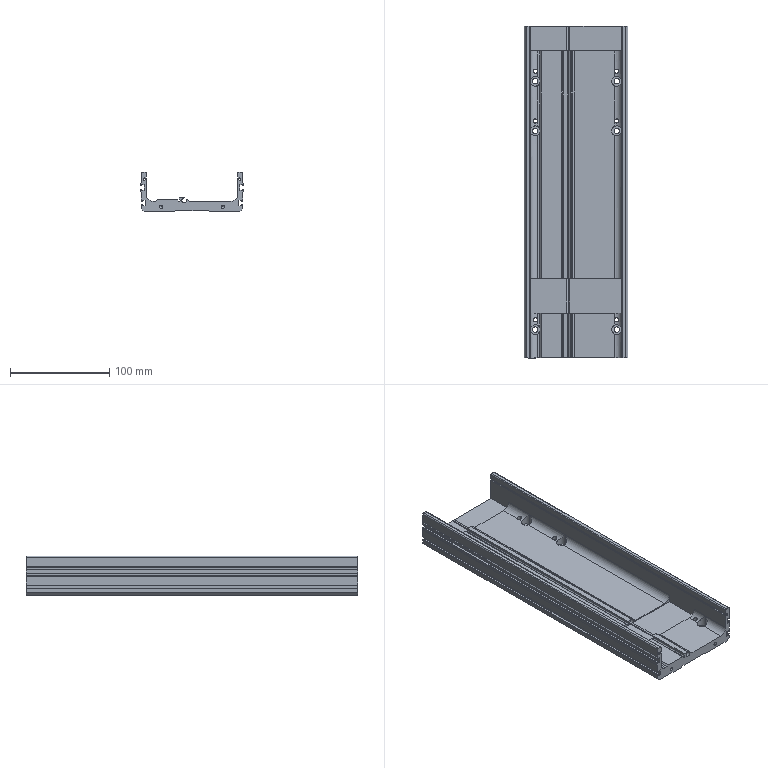Part | SolidWorks | features BaseBody 1 | 1 solid | 192 faces | box 104 x 334 x 40 mm | volume 423472 mm3 | plane 96 | cylinder 88 | cone 8 | commonest cylinder face diameters 4.2 x12 5.5 x12 10 x12 14 x10 1 x8 2 x8